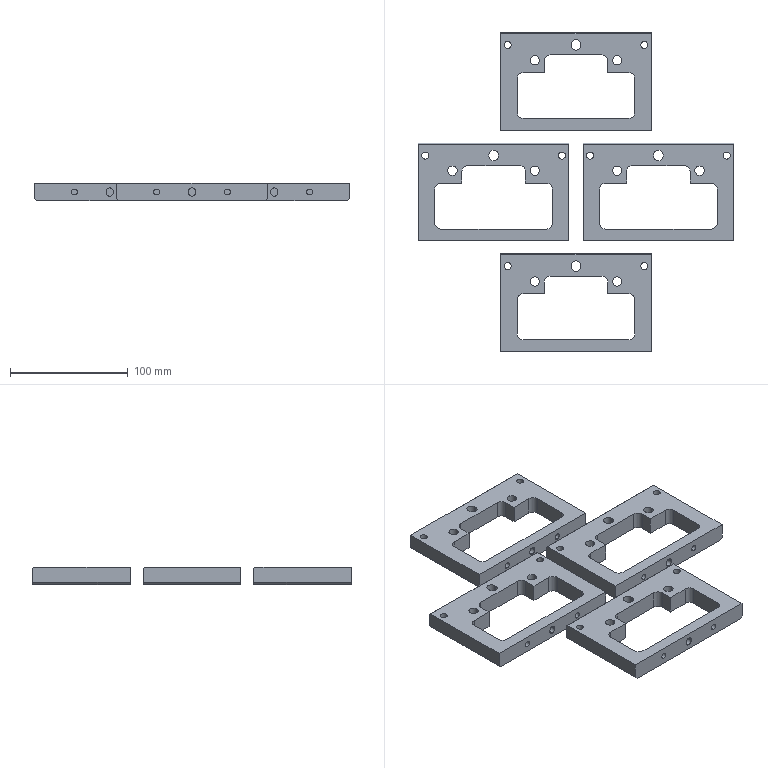NC program | NX | posted with a generic post | part box 268 x 271 x 15 mm
Lines 1 to 29 of 2286:
N10 G17 G21 G94 G90
(DRILLING_COPY_1 , TOOL : D6A45)
N12 T07 M6
N14 G54
N16 G17 G0 G90 X-30. Y0. B0. C0. S5000 M3
N18 G43 Z30. H7
N20 G94 G81 G98 Z-1. F250. R3.
N22 X0. Y0.5
N24 X30. Y0.
N26 G80
N28 G0 X30. Y0. Z30.
N30 M5
(DRILLING_COPY_COPY_1 , TOOL : 5.0ZT)
N32 T15 M6
N34 G54
N36 G17 G0 G90 X-30. Y0. B0. C0. S2000 M3
N38 G43 Z30. H15
N40 G94 G83 G98 Z-13.002 F200. Q2. R3.
N42 X0. Y0.5 Z-8.
N44 X30. Y0. Z-13.002
N46 G80
N48 G0 X30. Y0. Z30.
N50 M5